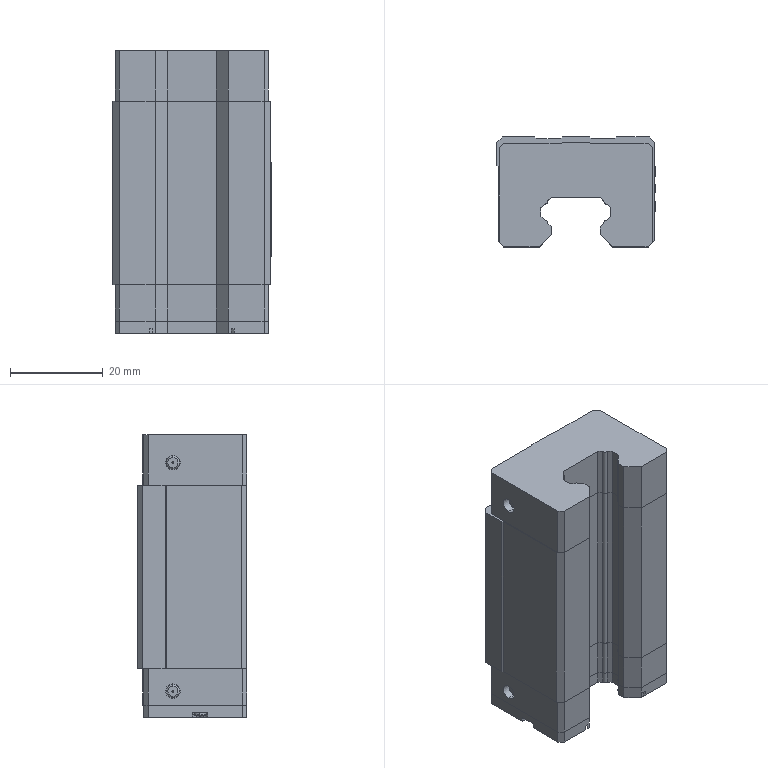Part | SolidWorks | features ICE 19, MirrorPattern 4, Chamfer 3, Extrusion 3, MirrorSolid 3, Fillet 2, Dome 1, RevCut 1, Revolution 1 | 4 solids | 1274 faces | box 34.1 x 23.6 x 60.875 mm | volume 38055 mm3 | plane 812 | spline 370 | cylinder 68 | torus 12 | cone 8 | sphere 4 | commonest cylinder face diameters 1.459 x24 3.15 x12 0.425 x8 3.2 x8 4 x8 2.638 x4